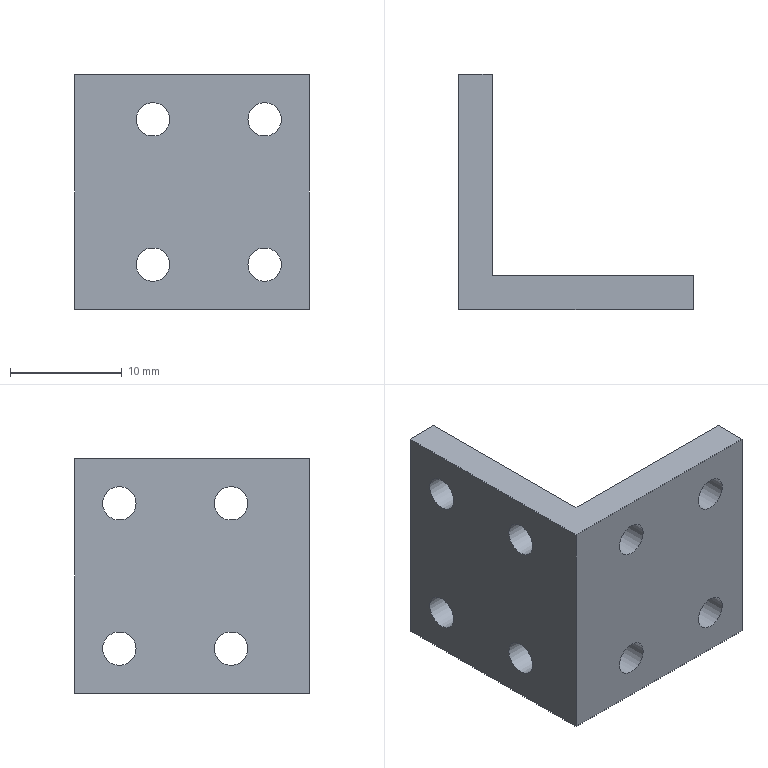Part | STEP file | 1-01.5 | 1 solid | 16 faces | box 21 x 21 x 21 mm | volume 2287 mm3 | plane 8 | cylinder 8 | commonest cylinder face diameters 3 x8
STEP:
#1=CARTESIAN_POINT('',(0.,0.,0.));
#2=DIRECTION('',(0.,0.,1.));
#3=DIRECTION('',(1.,0.,0.));
#4=AXIS2_PLACEMENT_3D('',#1,#2,#3);
#5=CARTESIAN_POINT('',(-3.,-10.5,-10.5));
#6=VERTEX_POINT('',#5);
#7=CARTESIAN_POINT('',(-3.,10.5,-10.5));
#8=VERTEX_POINT('',#7);
#9=CARTESIAN_POINT('',(-3.,-10.5,-10.5));
#10=DIRECTION('',(0.,1.,0.));
#11=VECTOR('',#10,1.);
#12=LINE('',#9,#11);
#13=CARTESIAN_POINT('',(-3.,0.,0.));
#14=DIRECTION('',(1.,0.,0.));
#15=DIRECTION('',(0.,1.,0.));
#16=AXIS2_PLACEMENT_3D('',#13,#14,#15);
#17=PLANE('',#16);
#18=CARTESIAN_POINT('',(-10.5,-10.5));
#19=DIRECTION('',(1.,0.));
#20=VECTOR('',#19,1.);
#21=LINE('',#18,#20);
#22=(GEOMETRIC_REPRESENTATION_CONTEXT(2)PARAMETRIC_REPRESENTATION_CONTEXT()REPRESENTATION_CONTEXT('',''));
#23=DEFINITIONAL_REPRESENTATION('',(#21),#22);
#24=PCURVE('',#17,#23);
#25=CARTESIAN_POINT('',(7.5,0.,-10.5));
#26=DIRECTION('',(0.,0.,1.));
#27=DIRECTION('',(0.,1.,0.));
#28=AXIS2_PLACEMENT_3D('',#25,#26,#27);
#29=PLANE('',#28);
#30=CARTESIAN_POINT('',(-10.5,10.5));
#31=DIRECTION('',(1.,0.));
#32=VECTOR('',#31,1.);
#33=LINE('',#30,#32);
#34=(GEOMETRIC_REPRESENTATION_CONTEXT(2)PARAMETRIC_REPRESENTATION_CONTEXT()REPRESENTATION_CONTEXT('',''));
#35=DEFINITIONAL_REPRESENTATION('',(#33),#34);
#36=PCURVE('',#29,#35);
#37=SURFACE_CURVE('',#12,(#24,#36),.PCURVE_S1.);
#38=EDGE_CURVE('',#6,#8,#37,.T.);
#39=ORIENTED_EDGE('',*,*,#38,.T.);
#40=CARTESIAN_POINT('',(-3.,10.5,10.5));
#41=VERTEX_POINT('',#40);
#42=CARTESIAN_POINT('',(-3.,10.5,-10.5));
#43=DIRECTION('',(0.,0.,1.));
#44=VECTOR('',#43,1.);
#45=LINE('',#42,#44);
#46=CARTESIAN_POINT('',(10.5,-10.5));
#47=DIRECTION('',(0.,1.));
#48=VECTOR('',#47,1.);
#49=LINE('',#46,#48);
#50=(GEOMETRIC_REPRESENTATION_CONTEXT(2)PARAMETRIC_REPRESENTATION_CONTEXT()REPRESENTATION_CONTEXT('',''));
#51=DEFINITIONAL_REPRESENTATION('',(#49),#50);
#52=PCURVE('',#17,#51);
#53=CARTESIAN_POINT('',(-1.5,10.5,0.));
#54=DIRECTION('',(0.,-1.,0.));
#55=DIRECTION('',(0.,0.,1.));
#56=AXIS2_PLACEMENT_3D('',#53,#54,#55);
#57=PLANE('',#56);
#58=CARTESIAN_POINT('',(-10.5,1.5));
#59=DIRECTION('',(1.,0.));
#60=VECTOR('',#59,1.);
#61=LINE('',#58,#60);
#62=(GEOMETRIC_REPRESENTATION_CONTEXT(2)PARAMETRIC_REPRESENTATION_CONTEXT()REPRESENTATION_CONTEXT('',''));
#63=DEFINITIONAL_REPRESENTATION('',(#61),#62);
#64=PCURVE('',#57,#63);
#65=SURFACE_CURVE('',#45,(#52,#64),.PCURVE_S1.);
#66=EDGE_CURVE('',#8,#41,#65,.T.);
#67=ORIENTED_EDGE('',*,*,#66,.T.);
#68=CARTESIAN_POINT('',(-3.,-10.5,10.5));
#69=VERTEX_POINT('',#68);
#70=CARTESIAN_POINT('',(-3.,10.5,10.5));
#71=DIRECTION('',(0.,-1.,0.));
#72=VECTOR('',#71,1.);
#73=LINE('',#70,#72);
#74=CARTESIAN_POINT('',(10.5,10.5));
#75=DIRECTION('',(-1.,0.));
#76=VECTOR('',#75,1.);
#77=LINE('',#74,#76);
#78=(GEOMETRIC_REPRESENTATION_CONTEXT(2)PARAMETRIC_REPRESENTATION_CONTEXT()REPRESENTATION_CONTEXT('',''));
#79=DEFINITIONAL_REPRESENTATION('',(#77),#78);
#80=PCURVE('',#17,#79);
#81=CARTESIAN_POINT('',(7.5,0.,10.5));
#82=DIRECTION('',(0.,0.,-1.));
#83=DIRECTION('',(0.,-1.,0.));
#84=AXIS2_PLACEMENT_3D('',#81,#82,#83);
#85=PLANE('',#84);
#86=CARTESIAN_POINT('',(-10.5,10.5));
#87=DIRECTION('',(1.,0.));
#88=VECTOR('',#87,1.);
#89=LINE('',#86,#88);
#90=(GEOMETRIC_REPRESENTATION_CONTEXT(2)PARAMETRIC_REPRESENTATION_CONTEXT()REPRESENTATION_CONTEXT('',''));
#91=DEFINITIONAL_REPRESENTATION('',(#89),#90);
#92=PCURVE('',#85,#91);
#93=SURFACE_CURVE('',#73,(#80,#92),.PCURVE_S1.);
#94=EDGE_CURVE('',#41,#69,#93,.T.);
#95=ORIENTED_EDGE('',*,*,#94,.T.);
#96=CARTESIAN_POINT('',(-3.,-10.5,10.5));
#97=DIRECTION('',(0.,0.,-1.));
#98=VECTOR('',#97,1.);
#99=LINE('',#96,#98);
#100=CARTESIAN_POINT('',(-10.5,10.5));
#101=DIRECTION('',(0.,-1.));
#102=VECTOR('',#101,1.);
#103=LINE('',#100,#102);
#104=(GEOMETRIC_REPRESENTATION_CONTEXT(2)PARAMETRIC_REPRESENTATION_CONTEXT()REPRESENTATION_CONTEXT('',''));
#105=DEFINITIONAL_REPRESENTATION('',(#103),#104);
#106=PCURVE('',#17,#105);
#107=CARTESIAN_POINT('',(9.525,-10.5,0.));
#108=DIRECTION('',(0.,1.,0.));
#109=DIRECTION('',(0.,0.,-1.));
#110=AXIS2_PLACEMENT_3D('',#107,#108,#109);
#111=PLANE('',#110);
#112=CARTESIAN_POINT('',(-10.5,12.525));
#113=DIRECTION('',(1.,0.));
#114=VECTOR('',#113,1.);
#115=LINE('',#112,#114);
#116=(GEOMETRIC_REPRESENTATION_CONTEXT(2)PARAMETRIC_REPRESENTATION_CONTEXT()REPRESENTATION_CONTEXT('',''));
#117=DEFINITIONAL_REPRESENTATION('',(#115),#116);
#118=PCURVE('',#111,#117);
#119=SURFACE_CURVE('',#99,(#106,#118),.PCURVE_S1.);
#120=EDGE_CURVE('',#69,#6,#119,.T.);
#121=ORIENTED_EDGE('',*,*,#120,.T.);
#122=EDGE_LOOP('',(#39,#67,#95,#121));
#123=FACE_BOUND('',#122,.F.);
#124=CARTESIAN_POINT('',(-3.,8.,6.5));
#125=VERTEX_POINT('',#124);
#126=CARTESIAN_POINT('',(-3.,6.5,6.5));
#127=DIRECTION('',(-1.,0.,0.));
#128=DIRECTION('',(0.,1.,0.));
#129=AXIS2_PLACEMENT_3D('',#126,#127,#128);
#130=CIRCLE('',#129,1.5);
#131=CARTESIAN_POINT('',(8.,6.5));
#132=CARTESIAN_POINT('',(8.,3.902));
#133=CARTESIAN_POINT('',(5.75,5.201));
#134=CARTESIAN_POINT('',(3.5,6.5));
#135=CARTESIAN_POINT('',(5.75,7.799));
#136=CARTESIAN_POINT('',(8.,9.098));
#137=CARTESIAN_POINT('',(8.,6.5));
#138=(BOUNDED_CURVE()B_SPLINE_CURVE(2,(#131,#132,#133,#134,#135,#136,#137),.UNSPECIFIED.,.T.,.F.)B_SPLINE_CURVE_WITH_KNOTS((1,2,2,2,2,1),(-2.094,0.,2.094,4.189,6.283,8.378),.UNSPECIFIED.)CURVE()GEOMETRIC_REPRESENTATION_ITEM()RATIONAL_B_SPLINE_CURVE((1.,0.5,1.,0.5,1.,0.5,1.))REPRESENTATION_ITEM(''));
#139=(GEOMETRIC_REPRESENTATION_CONTEXT(2)PARAMETRIC_REPRESENTATION_CONTEXT()REPRESENTATION_CONTEXT('',''));
#140=DEFINITIONAL_REPRESENTATION('',(#138),#139);
#141=PCURVE('',#17,#140);
#142=CARTESIAN_POINT('',(0.,6.5,6.5));
#143=DIRECTION('',(-1.,0.,0.));
#144=DIRECTION('',(0.,1.,0.));
#145=AXIS2_PLACEMENT_3D('',#142,#143,#144);
#146=CYLINDRICAL_SURFACE('',#145,1.5);
#147=CARTESIAN_POINT('',(0.,3.));
#148=DIRECTION('',(1.,0.));
#149=VECTOR('',#148,1.);
#150=LINE('',#147,#149);
#151=(GEOMETRIC_REPRESENTATION_CONTEXT(2)PARAMETRIC_REPRESENTATION_CONTEXT()REPRESENTATION_CONTEXT('',''));
#152=DEFINITIONAL_REPRESENTATION('',(#150),#151);
#153=PCURVE('',#146,#152);
#154=SURFACE_CURVE('',#130,(#141,#153),.PCURVE_S1.);
#155=EDGE_CURVE('',#125,#125,#154,.T.);
#156=ORIENTED_EDGE('',*,*,#155,.T.);
#157=EDGE_LOOP('',(#156));
#158=FACE_BOUND('',#157,.F.);
#159=CARTESIAN_POINT('',(-3.,8.,-6.5));
#160=VERTEX_POINT('',#159);
#161=CARTESIAN_POINT('',(-3.,6.5,-6.5));
#162=DIRECTION('',(-1.,0.,0.));
#163=DIRECTION('',(0.,1.,0.));
#164=AXIS2_PLACEMENT_3D('',#161,#162,#163);
#165=CIRCLE('',#164,1.5);
#166=CARTESIAN_POINT('',(8.,-6.5));
#167=CARTESIAN_POINT('',(8.,-9.098));
#168=CARTESIAN_POINT('',(5.75,-7.799));
#169=CARTESIAN_POINT('',(3.5,-6.5));
#170=CARTESIAN_POINT('',(5.75,-5.201));
#171=CARTESIAN_POINT('',(8.,-3.902));
#172=CARTESIAN_POINT('',(8.,-6.5));
#173=(BOUNDED_CURVE()B_SPLINE_CURVE(2,(#166,#167,#168,#169,#170,#171,#172),.UNSPECIFIED.,.T.,.F.)B_SPLINE_CURVE_WITH_KNOTS((1,2,2,2,2,1),(-2.094,0.,2.094,4.189,6.283,8.378),.UNSPECIFIED.)CURVE()GEOMETRIC_REPRESENTATION_ITEM()RATIONAL_B_SPLINE_CURVE((1.,0.5,1.,0.5,1.,0.5,1.))REPRESENTATION_ITEM(''));
#174=(GEOMETRIC_REPRESENTATION_CONTEXT(2)PARAMETRIC_REPRESENTATION_CONTEXT()REPRESENTATION_CONTEXT('',''));
#175=DEFINITIONAL_REPRESENTATION('',(#173),#174);
#176=PCURVE('',#17,#175);
#177=CARTESIAN_POINT('',(0.,6.5,-6.5));
#178=DIRECTION('',(-1.,0.,0.));
#179=DIRECTION('',(0.,1.,0.));
#180=AXIS2_PLACEMENT_3D('',#177,#178,#179);
#181=CYLINDRICAL_SURFACE('',#180,1.5);
#182=CARTESIAN_POINT('',(0.,3.));
#183=DIRECTION('',(1.,0.));
#184=VECTOR('',#183,1.);
#185=LINE('',#182,#184);
#186=(GEOMETRIC_REPRESENTATION_CONTEXT(2)PARAMETRIC_REPRESENTATION_CONTEXT()REPRESENTATION_CONTEXT('',''));
#187=DEFINITIONAL_REPRESENTATION('',(#185),#186);
#188=PCURVE('',#181,#187);
#189=SURFACE_CURVE('',#165,(#176,#188),.PCURVE_S1.);
#190=EDGE_CURVE('',#160,#160,#189,.T.);
#191=ORIENTED_EDGE('',*,*,#190,.T.);
#192=EDGE_LOOP('',(#191));
#193=FACE_BOUND('',#192,.F.);
#194=CARTESIAN_POINT('',(-3.,-2.,-6.5));
#195=VERTEX_POINT('',#194);
#196=CARTESIAN_POINT('',(-3.,-3.5,-6.5));
#197=DIRECTION('',(-1.,0.,0.));
#198=DIRECTION('',(0.,1.,0.));
#199=AXIS2_PLACEMENT_3D('',#196,#197,#198);
#200=CIRCLE('',#199,1.5);
#201=CARTESIAN_POINT('',(-2.,-6.5));
#202=CARTESIAN_POINT('',(-2.,-9.098));
#203=CARTESIAN_POINT('',(-4.25,-7.799));
#204=CARTESIAN_POINT('',(-6.5,-6.5));
#205=CARTESIAN_POINT('',(-4.25,-5.201));
#206=CARTESIAN_POINT('',(-2.,-3.902));
#207=CARTESIAN_POINT('',(-2.,-6.5));
#208=(BOUNDED_CURVE()B_SPLINE_CURVE(2,(#201,#202,#203,#204,#205,#206,#207),.UNSPECIFIED.,.T.,.F.)B_SPLINE_CURVE_WITH_KNOTS((1,2,2,2,2,1),(-2.094,0.,2.094,4.189,6.283,8.378),.UNSPECIFIED.)CURVE()GEOMETRIC_REPRESENTATION_ITEM()RATIONAL_B_SPLINE_CURVE((1.,0.5,1.,0.5,1.,0.5,1.))REPRESENTATION_ITEM(''));
#209=(GEOMETRIC_REPRESENTATION_CONTEXT(2)PARAMETRIC_REPRESENTATION_CONTEXT()REPRESENTATION_CONTEXT('',''));
#210=DEFINITIONAL_REPRESENTATION('',(#208),#209);
#211=PCURVE('',#17,#210);
#212=CARTESIAN_POINT('',(0.,-3.5,-6.5));
#213=DIRECTION('',(-1.,0.,0.));
#214=DIRECTION('',(0.,1.,0.));
#215=AXIS2_PLACEMENT_3D('',#212,#213,#214);
#216=CYLINDRICAL_SURFACE('',#215,1.5);
#217=CARTESIAN_POINT('',(0.,3.));
#218=DIRECTION('',(1.,0.));
#219=VECTOR('',#218,1.);
#220=LINE('',#217,#219);
#221=(GEOMETRIC_REPRESENTATION_CONTEXT(2)PARAMETRIC_REPRESENTATION_CONTEXT()REPRESENTATION_CONTEXT('',''));
#222=DEFINITIONAL_REPRESENTATION('',(#220),#221);
#223=PCURVE('',#216,#222);
#224=SURFACE_CURVE('',#200,(#211,#223),.PCURVE_S1.);
#225=EDGE_CURVE('',#195,#195,#224,.T.);
#226=ORIENTED_EDGE('',*,*,#225,.T.);
#227=EDGE_LOOP('',(#226));
#228=FACE_BOUND('',#227,.F.);
#229=CARTESIAN_POINT('',(-3.,-2.,6.5));
#230=VERTEX_POINT('',#229);
#231=CARTESIAN_POINT('',(-3.,-3.5,6.5));
#232=DIRECTION('',(-1.,0.,0.));
#233=DIRECTION('',(0.,1.,0.));
#234=AXIS2_PLACEMENT_3D('',#231,#232,#233);
#235=CIRCLE('',#234,1.5);
#236=CARTESIAN_POINT('',(-2.,6.5));
#237=CARTESIAN_POINT('',(-2.,3.902));
#238=CARTESIAN_POINT('',(-4.25,5.201));
#239=CARTESIAN_POINT('',(-6.5,6.5));
#240=CARTESIAN_POINT('',(-4.25,7.799));
#241=CARTESIAN_POINT('',(-2.,9.098));
#242=CARTESIAN_POINT('',(-2.,6.5));
#243=(BOUNDED_CURVE()B_SPLINE_CURVE(2,(#236,#237,#238,#239,#240,#241,#242),.UNSPECIFIED.,.T.,.F.)B_SPLINE_CURVE_WITH_KNOTS((1,2,2,2,2,1),(-2.094,0.,2.094,4.189,6.283,8.378),.UNSPECIFIED.)CURVE()GEOMETRIC_REPRESENTATION_ITEM()RATIONAL_B_SPLINE_CURVE((1.,0.5,1.,0.5,1.,0.5,1.))REPRESENTATION_ITEM(''));
#244=(GEOMETRIC_REPRESENTATION_CONTEXT(2)PARAMETRIC_REPRESENTATION_CONTEXT()REPRESENTATION_CONTEXT('',''));
#245=DEFINITIONAL_REPRESENTATION('',(#243),#244);
#246=PCURVE('',#17,#245);
#247=CARTESIAN_POINT('',(0.,-3.5,6.5));
#248=DIRECTION('',(-1.,0.,0.));
#249=DIRECTION('',(0.,1.,0.));
#250=AXIS2_PLACEMENT_3D('',#247,#248,#249);
#251=CYLINDRICAL_SURFACE('',#250,1.5);
#252=CARTESIAN_POINT('',(0.,3.));
#253=DIRECTION('',(1.,0.));
#254=VECTOR('',#253,1.);
#255=LINE('',#252,#254);
#256=(GEOMETRIC_REPRESENTATION_CONTEXT(2)PARAMETRIC_REPRESENTATION_CONTEXT()REPRESENTATION_CONTEXT('',''));
#257=DEFINITIONAL_REPRESENTATION('',(#255),#256);
#258=PCURVE('',#251,#257);
#259=SURFACE_CURVE('',#235,(#246,#258),.PCURVE_S1.);
#260=EDGE_CURVE('',#230,#230,#259,.T.);
#261=ORIENTED_EDGE('',*,*,#260,.T.);
#262=EDGE_LOOP('',(#261));
#263=FACE_BOUND('',#262,.F.);
#264=ADVANCED_FACE('',(#123,#158,#193,#228,#263),#17,.F.);
#265=CARTESIAN_POINT('',(0.,-7.5,-10.5));
#266=VERTEX_POINT('',#265);
#267=CARTESIAN_POINT('',(0.,10.5,-10.5));
#268=VERTEX_POINT('',#267);
#269=CARTESIAN_POINT('',(0.,-7.5,-10.5));
#270=DIRECTION('',(0.,1.,0.));
#271=VECTOR('',#270,1.);
#272=LINE('',#269,#271);
#273=CARTESIAN_POINT('',(-7.5,7.5));
#274=DIRECTION('',(1.,0.));
#275=VECTOR('',#274,1.);
#276=LINE('',#273,#275);
#277=(GEOMETRIC_REPRESENTATION_CONTEXT(2)PARAMETRIC_REPRESENTATION_CONTEXT()REPRESENTATION_CONTEXT('',''));
#278=DEFINITIONAL_REPRESENTATION('',(#276),#277);
#279=PCURVE('',#29,#278);
#280=CARTESIAN_POINT('',(0.,0.,0.));
#281=DIRECTION('',(1.,0.,0.));
#282=DIRECTION('',(0.,1.,0.));
#283=AXIS2_PLACEMENT_3D('',#280,#281,#282);
#284=PLANE('',#283);
#285=CARTESIAN_POINT('',(-7.5,-10.5));
#286=DIRECTION('',(1.,0.));
#287=VECTOR('',#286,1.);
#288=LINE('',#285,#287);
#289=(GEOMETRIC_REPRESENTATION_CONTEXT(2)PARAMETRIC_REPRESENTATION_CONTEXT()REPRESENTATION_CONTEXT('',''));
#290=DEFINITIONAL_REPRESENTATION('',(#288),#289);
#291=PCURVE('',#284,#290);
#292=SURFACE_CURVE('',#272,(#279,#291),.PCURVE_S1.);
#293=EDGE_CURVE('',#266,#268,#292,.T.);
#294=ORIENTED_EDGE('',*,*,#293,.T.);
#295=CARTESIAN_POINT('',(0.,10.5,-10.5));
#296=DIRECTION('',(-1.,0.,0.));
#297=VECTOR('',#296,1.);
#298=LINE('',#295,#297);
#299=CARTESIAN_POINT('',(10.5,7.5));
#300=DIRECTION('',(0.,1.));
#301=VECTOR('',#300,1.);
#302=LINE('',#299,#301);
#303=(GEOMETRIC_REPRESENTATION_CONTEXT(2)PARAMETRIC_REPRESENTATION_CONTEXT()REPRESENTATION_CONTEXT('',''));
#304=DEFINITIONAL_REPRESENTATION('',(#302),#303);
#305=PCURVE('',#29,#304);
#306=CARTESIAN_POINT('',(-10.5,-1.5));
#307=DIRECTION('',(0.,1.));
#308=VECTOR('',#307,1.);
#309=LINE('',#306,#308);
#310=(GEOMETRIC_REPRESENTATION_CONTEXT(2)PARAMETRIC_REPRESENTATION_CONTEXT()REPRESENTATION_CONTEXT('',''));
#311=DEFINITIONAL_REPRESENTATION('',(#309),#310);
#312=PCURVE('',#57,#311);
#313=SURFACE_CURVE('',#298,(#305,#312),.PCURVE_S1.);
#314=EDGE_CURVE('',#268,#8,#313,.T.);
#315=ORIENTED_EDGE('',*,*,#314,.T.);
#316=ORIENTED_EDGE('',*,*,#38,.F.);
#317=CARTESIAN_POINT('',(18.,-10.5,-10.5));
#318=VERTEX_POINT('',#317);
#319=CARTESIAN_POINT('',(18.,-10.5,-10.5));
#320=DIRECTION('',(-1.,0.,0.));
#321=VECTOR('',#320,1.);
#322=LINE('',#319,#321);
#323=CARTESIAN_POINT('',(-10.5,-10.5));
#324=DIRECTION('',(0.,1.));
#325=VECTOR('',#324,1.);
#326=LINE('',#323,#325);
#327=(GEOMETRIC_REPRESENTATION_CONTEXT(2)PARAMETRIC_REPRESENTATION_CONTEXT()REPRESENTATION_CONTEXT('',''));
#328=DEFINITIONAL_REPRESENTATION('',(#326),#327);
#329=PCURVE('',#29,#328);
#330=CARTESIAN_POINT('',(10.5,-8.475));
#331=DIRECTION('',(0.,1.));
#332=VECTOR('',#331,1.);
#333=LINE('',#330,#332);
#334=(GEOMETRIC_REPRESENTATION_CONTEXT(2)PARAMETRIC_REPRESENTATION_CONTEXT()REPRESENTATION_CONTEXT('',''));
#335=DEFINITIONAL_REPRESENTATION('',(#333),#334);
#336=PCURVE('',#111,#335);
#337=SURFACE_CURVE('',#322,(#329,#336),.PCURVE_S1.);
#338=EDGE_CURVE('',#318,#6,#337,.T.);
#339=ORIENTED_EDGE('',*,*,#338,.F.);
#340=CARTESIAN_POINT('',(18.,-7.5,-10.5));
#341=VERTEX_POINT('',#340);
#342=CARTESIAN_POINT('',(18.,-10.5,-10.5));
#343=DIRECTION('',(0.,1.,0.));
#344=VECTOR('',#343,1.);
#345=LINE('',#342,#344);
#346=CARTESIAN_POINT('',(-10.5,-10.5));
#347=DIRECTION('',(1.,0.));
#348=VECTOR('',#347,1.);
#349=LINE('',#346,#348);
#350=(GEOMETRIC_REPRESENTATION_CONTEXT(2)PARAMETRIC_REPRESENTATION_CONTEXT()REPRESENTATION_CONTEXT('',''));
#351=DEFINITIONAL_REPRESENTATION('',(#349),#350);
#352=PCURVE('',#29,#351);
#353=CARTESIAN_POINT('',(18.,-9.,0.));
#354=DIRECTION('',(-1.,0.,0.));
#355=DIRECTION('',(0.,0.,1.));
#356=AXIS2_PLACEMENT_3D('',#353,#354,#355);
#357=PLANE('',#356);
#358=CARTESIAN_POINT('',(-10.5,-1.5));
#359=DIRECTION('',(0.,1.));
#360=VECTOR('',#359,1.);
#361=LINE('',#358,#360);
#362=(GEOMETRIC_REPRESENTATION_CONTEXT(2)PARAMETRIC_REPRESENTATION_CONTEXT()REPRESENTATION_CONTEXT('',''));
#363=DEFINITIONAL_REPRESENTATION('',(#361),#362);
#364=PCURVE('',#357,#363);
#365=SURFACE_CURVE('',#345,(#352,#364),.PCURVE_S1.);
#366=EDGE_CURVE('',#318,#341,#365,.T.);
#367=ORIENTED_EDGE('',*,*,#366,.T.);
#368=CARTESIAN_POINT('',(0.,-7.5,-10.5));
#369=DIRECTION('',(1.,0.,0.));
#370=VECTOR('',#369,1.);
#371=LINE('',#368,#370);
#372=CARTESIAN_POINT('',(-7.5,7.5));
#373=DIRECTION('',(0.,-1.));
#374=VECTOR('',#373,1.);
#375=LINE('',#372,#374);
#376=(GEOMETRIC_REPRESENTATION_CONTEXT(2)PARAMETRIC_REPRESENTATION_CONTEXT()REPRESENTATION_CONTEXT('',''));
#377=DEFINITIONAL_REPRESENTATION('',(#375),#376);
#378=PCURVE('',#29,#377);
#379=CARTESIAN_POINT('',(10.5,-7.5,0.));
#380=DIRECTION('',(0.,-1.,0.));
#381=DIRECTION('',(1.,0.,0.));
#382=AXIS2_PLACEMENT_3D('',#379,#380,#381);
#383=PLANE('',#382);
#384=CARTESIAN_POINT('',(-10.5,-10.5));
#385=DIRECTION('',(1.,0.));
#386=VECTOR('',#385,1.);
#387=LINE('',#384,#386);
#388=(GEOMETRIC_REPRESENTATION_CONTEXT(2)PARAMETRIC_REPRESENTATION_CONTEXT()REPRESENTATION_CONTEXT('',''));
#389=DEFINITIONAL_REPRESENTATION('',(#387),#388);
#390=PCURVE('',#383,#389);
#391=SURFACE_CURVE('',#371,(#378,#390),.PCURVE_S1.);
#392=EDGE_CURVE('',#266,#341,#391,.T.);
#393=ORIENTED_EDGE('',*,*,#392,.F.);
#394=EDGE_LOOP('',(#294,#315,#316,#339,#367,#393));
#395=FACE_BOUND('',#394,.F.);
#396=ADVANCED_FACE('',(#395),#29,.F.);
#397=CARTESIAN_POINT('',(0.,10.5,10.5));
#398=VERTEX_POINT('',#397);
#399=CARTESIAN_POINT('',(0.,10.5,-10.5));
#400=DIRECTION('',(0.,0.,1.));
#401=VECTOR('',#400,1.);
#402=LINE('',#399,#401);
#403=CARTESIAN_POINT('',(-10.5,-1.5));
#404=DIRECTION('',(1.,0.));
#405=VECTOR('',#404,1.);
#406=LINE('',#403,#405);
#407=(GEOMETRIC_REPRESENTATION_CONTEXT(2)PARAMETRIC_REPRESENTATION_CONTEXT()REPRESENTATION_CONTEXT('',''));
#408=DEFINITIONAL_REPRESENTATION('',(#406),#407);
#409=PCURVE('',#57,#408);
#410=CARTESIAN_POINT('',(10.5,-10.5));
#411=DIRECTION('',(0.,1.));
#412=VECTOR('',#411,1.);
#413=LINE('',#410,#412);
#414=(GEOMETRIC_REPRESENTATION_CONTEXT(2)PARAMETRIC_REPRESENTATION_CONTEXT()REPRESENTATION_CONTEXT('',''));
#415=DEFINITIONAL_REPRESENTATION('',(#413),#414);
#416=PCURVE('',#284,#415);
#417=SURFACE_CURVE('',#402,(#409,#416),.PCURVE_S1.);
#418=EDGE_CURVE('',#268,#398,#417,.T.);
#419=ORIENTED_EDGE('',*,*,#418,.T.);
#420=CARTESIAN_POINT('',(0.,10.5,10.5));
#421=DIRECTION('',(-1.,0.,0.));
#422=VECTOR('',#421,1.);
#423=LINE('',#420,#422);
#424=CARTESIAN_POINT('',(10.5,-1.5));
#425=DIRECTION('',(0.,1.));
#426=VECTOR('',#425,1.);
#427=LINE('',#424,#426);
#428=(GEOMETRIC_REPRESENTATION_CONTEXT(2)PARAMETRIC_REPRESENTATION_CONTEXT()REPRESENTATION_CONTEXT('',''));
#429=DEFINITIONAL_REPRESENTATION('',(#427),#428);
#430=PCURVE('',#57,#429);
#431=CARTESIAN_POINT('',(-10.5,7.5));
#432=DIRECTION('',(0.,1.));
#433=VECTOR('',#432,1.);
#434=LINE('',#431,#433);
#435=(GEOMETRIC_REPRESENTATION_CONTEXT(2)PARAMETRIC_REPRESENTATION_CONTEXT()REPRESENTATION_CONTEXT('',''));
#436=DEFINITIONAL_REPRESENTATION('',(#434),#435);
#437=PCURVE('',#85,#436);
#438=SURFACE_CURVE('',#423,(#430,#437),.PCURVE_S1.);
#439=EDGE_CURVE('',#398,#41,#438,.T.);
#440=ORIENTED_EDGE('',*,*,#439,.T.);
#441=ORIENTED_EDGE('',*,*,#66,.F.);
#442=ORIENTED_EDGE('',*,*,#314,.F.);
#443=EDGE_LOOP('',(#419,#440,#441,#442));
#444=FACE_BOUND('',#443,.F.);
#445=ADVANCED_FACE('',(#444),#57,.F.);
#446=ORIENTED_EDGE('',*,*,#94,.F.);
#447=ORIENTED_EDGE('',*,*,#439,.F.);
#448=CARTESIAN_POINT('',(0.,-7.5,10.5));
#449=VERTEX_POINT('',#448);
#450=CARTESIAN_POINT('',(0.,10.5,10.5));
#451=DIRECTION('',(0.,-1.,0.));
#452=VECTOR('',#451,1.);
#453=LINE('',#450,#452);
#454=CARTESIAN_POINT('',(-10.5,7.5));
#455=DIRECTION('',(1.,0.));
#456=VECTOR('',#455,1.);
#457=LINE('',#454,#456);
#458=(GEOMETRIC_REPRESENTATION_CONTEXT(2)PARAMETRIC_REPRESENTATION_CONTEXT()REPRESENTATION_CONTEXT('',''));
#459=DEFINITIONAL_REPRESENTATION('',(#457),#458);
#460=PCURVE('',#85,#459);
#461=CARTESIAN_POINT('',(10.5,10.5));
#462=DIRECTION('',(-1.,0.));
#463=VECTOR('',#462,1.);
#464=LINE('',#461,#463);
#465=(GEOMETRIC_REPRESENTATION_CONTEXT(2)PARAMETRIC_REPRESENTATION_CONTEXT()REPRESENTATION_CONTEXT('',''));
#466=DEFINITIONAL_REPRESENTATION('',(#464),#465);
#467=PCURVE('',#284,#466);
#468=SURFACE_CURVE('',#453,(#460,#467),.PCURVE_S1.);
#469=EDGE_CURVE('',#398,#449,#468,.T.);
#470=ORIENTED_EDGE('',*,*,#469,.T.);
#471=CARTESIAN_POINT('',(18.,-7.5,10.5));
#472=VERTEX_POINT('',#471);
#473=CARTESIAN_POINT('',(18.,-7.5,10.5));
#474=DIRECTION('',(-1.,0.,0.));
#475=VECTOR('',#474,1.);
#476=LINE('',#473,#475);
#477=CARTESIAN_POINT('',(7.5,-10.5));
#478=DIRECTION('',(0.,1.));
#479=VECTOR('',#478,1.);
#480=LINE('',#477,#479);
#481=(GEOMETRIC_REPRESENTATION_CONTEXT(2)PARAMETRIC_REPRESENTATION_CONTEXT()REPRESENTATION_CONTEXT('',''));
#482=DEFINITIONAL_REPRESENTATION('',(#480),#481);
#483=PCURVE('',#85,#482);
#484=CARTESIAN_POINT('',(7.5,10.5));
#485=DIRECTION('',(-1.,0.));
#486=VECTOR('',#485,1.);
#487=LINE('',#484,#486);
#488=(GEOMETRIC_REPRESENTATION_CONTEXT(2)PARAMETRIC_REPRESENTATION_CONTEXT()REPRESENTATION_CONTEXT('',''));
#489=DEFINITIONAL_REPRESENTATION('',(#487),#488);
#490=PCURVE('',#383,#489);
#491=SURFACE_CURVE('',#476,(#483,#490),.PCURVE_S1.);
#492=EDGE_CURVE('',#472,#449,#491,.T.);
#493=ORIENTED_EDGE('',*,*,#492,.F.);
#494=CARTESIAN_POINT('',(18.,-10.5,10.5));
#495=VERTEX_POINT('',#494);
#496=CARTESIAN_POINT('',(18.,-10.5,10.5));
#497=DIRECTION('',(0.,1.,0.));
#498=VECTOR('',#497,1.);
#499=LINE('',#496,#498);
#500=CARTESIAN_POINT('',(10.5,-10.5));
#501=DIRECTION('',(-1.,0.));
#502=VECTOR('',#501,1.);
#503=LINE('',#500,#502);
#504=(GEOMETRIC_REPRESENTATION_CONTEXT(2)PARAMETRIC_REPRESENTATION_CONTEXT()REPRESENTATION_CONTEXT('',''));
#505=DEFINITIONAL_REPRESENTATION('',(#503),#504);
#506=PCURVE('',#85,#505);
#507=CARTESIAN_POINT('',(10.5,-1.5));
#508=DIRECTION('',(0.,1.));
#509=VECTOR('',#508,1.);
#510=LINE('',#507,#509);
#511=(GEOMETRIC_REPRESENTATION_CONTEXT(2)PARAMETRIC_REPRESENTATION_CONTEXT()REPRESENTATION_CONTEXT('',''));
#512=DEFINITIONAL_REPRESENTATION('',(#510),#511);
#513=PCURVE('',#357,#512);
#514=SURFACE_CURVE('',#499,(#506,#513),.PCURVE_S1.);
#515=EDGE_CURVE('',#495,#472,#514,.T.);
#516=ORIENTED_EDGE('',*,*,#515,.F.);
#517=CARTESIAN_POINT('',(-3.,-10.5,10.5));
#518=DIRECTION('',(1.,0.,0.));
#519=VECTOR('',#518,1.);
#520=LINE('',#517,#519);
#521=CARTESIAN_POINT('',(10.5,10.5));
#522=DIRECTION('',(0.,-1.));
#523=VECTOR('',#522,1.);
#524=LINE('',#521,#523);
#525=(GEOMETRIC_REPRESENTATION_CONTEXT(2)PARAMETRIC_REPRESENTATION_CONTEXT()REPRESENTATION_CONTEXT('',''));
#526=DEFINITIONAL_REPRESENTATION('',(#524),#525);
#527=PCURVE('',#85,#526);
#528=CARTESIAN_POINT('',(-10.5,12.525));
#529=DIRECTION('',(0.,-1.));
#530=VECTOR('',#529,1.);
#531=LINE('',#528,#530);
#532=(GEOMETRIC_REPRESENTATION_CONTEXT(2)PARAMETRIC_REPRESENTATION_CONTEXT()REPRESENTATION_CONTEXT('',''));
#533=DEFINITIONAL_REPRESENTATION('',(#531),#532);
#534=PCURVE('',#111,#533);
#535=SURFACE_CURVE('',#520,(#527,#534),.PCURVE_S1.);
#536=EDGE_CURVE('',#69,#495,#535,.T.);
#537=ORIENTED_EDGE('',*,*,#536,.F.);
#538=EDGE_LOOP('',(#446,#447,#470,#493,#516,#537));
#539=FACE_BOUND('',#538,.F.);
#540=ADVANCED_FACE('',(#539),#85,.F.);
#541=ORIENTED_EDGE('',*,*,#120,.F.);
#542=ORIENTED_EDGE('',*,*,#536,.T.);
#543=CARTESIAN_POINT('',(18.,-10.5,-10.5));
#544=DIRECTION('',(0.,0.,1.));
#545=VECTOR('',#544,1.);
#546=LINE('',#543,#545);
#547=CARTESIAN_POINT('',(10.5,-8.475));
#548=DIRECTION('',(-1.,0.));
#549=VECTOR('',#548,1.);
#550=LINE('',#547,#549);
#551=(GEOMETRIC_REPRESENTATION_CONTEXT(2)PARAMETRIC_REPRESENTATION_CONTEXT()REPRESENTATION_CONTEXT('',''));
#552=DEFINITIONAL_REPRESENTATION('',(#550),#551);
#553=PCURVE('',#111,#552);
#554=CARTESIAN_POINT('',(-10.5,-1.5));
#555=DIRECTION('',(1.,0.));
#556=VECTOR('',#555,1.);
#557=LINE('',#554,#556);
#558=(GEOMETRIC_REPRESENTATION_CONTEXT(2)PARAMETRIC_REPRESENTATION_CONTEXT()REPRESENTATION_CONTEXT('',''));
#559=DEFINITIONAL_REPRESENTATION('',(#557),#558);
#560=PCURVE('',#357,#559);
#561=SURFACE_CURVE('',#546,(#553,#560),.PCURVE_S1.);
#562=EDGE_CURVE('',#318,#495,#561,.T.);
#563=ORIENTED_EDGE('',*,*,#562,.F.);
#564=ORIENTED_EDGE('',*,*,#338,.T.);
#565=EDGE_LOOP('',(#541,#542,#563,#564));
#566=FACE_BOUND('',#565,.F.);
#567=CARTESIAN_POINT('',(5.5,-10.5,-6.5));
#568=VERTEX_POINT('',#567);
#569=CARTESIAN_POINT('',(4.,-10.5,-6.5));
#570=DIRECTION('',(0.,1.,0.));
#571=DIRECTION('',(1.,0.,0.));
#572=AXIS2_PLACEMENT_3D('',#569,#570,#571);
#573=CIRCLE('',#572,1.5);
#574=CARTESIAN_POINT('',(6.5,5.525));
#575=DIRECTION('',(0.,-1.));
#576=AXIS2_PLACEMENT_2D('',#574,#575);
#577=CIRCLE('',#576,1.5);
#578=(GEOMETRIC_REPRESENTATION_CONTEXT(2)PARAMETRIC_REPRESENTATION_CONTEXT()REPRESENTATION_CONTEXT('',''));
#579=DEFINITIONAL_REPRESENTATION('',(#577),#578);
#580=PCURVE('',#111,#579);
#581=CARTESIAN_POINT('',(4.,-10.5,-6.5));
#582=DIRECTION('',(0.,1.,0.));
#583=DIRECTION('',(1.,0.,0.));
#584=AXIS2_PLACEMENT_3D('',#581,#582,#583);
#585=CYLINDRICAL_SURFACE('',#584,1.5);
#586=CARTESIAN_POINT('',(0.,0.));
#587=DIRECTION('',(1.,0.));
#588=VECTOR('',#587,1.);
#589=LINE('',#586,#588);
#590=(GEOMETRIC_REPRESENTATION_CONTEXT(2)PARAMETRIC_REPRESENTATION_CONTEXT()REPRESENTATION_CONTEXT('',''));
#591=DEFINITIONAL_REPRESENTATION('',(#589),#590);
#592=PCURVE('',#585,#591);
#593=SURFACE_CURVE('',#573,(#580,#592),.PCURVE_S1.);
#594=EDGE_CURVE('',#568,#568,#593,.T.);
#595=ORIENTED_EDGE('',*,*,#594,.F.);
#596=EDGE_LOOP('',(#595));
#597=FACE_BOUND('',#596,.F.);
#598=CARTESIAN_POINT('',(5.5,-10.5,6.5));
#599=VERTEX_POINT('',#598);
#600=CARTESIAN_POINT('',(4.,-10.5,6.5));
#601=DIRECTION('',(0.,1.,0.));
#602=DIRECTION('',(1.,0.,0.));
#603=AXIS2_PLACEMENT_3D('',#600,#601,#602);
#604=CIRCLE('',#603,1.5);
#605=CARTESIAN_POINT('',(-6.5,5.525));
#606=DIRECTION('',(0.,-1.));
#607=AXIS2_PLACEMENT_2D('',#605,#606);
#608=CIRCLE('',#607,1.5);
#609=(GEOMETRIC_REPRESENTATION_CONTEXT(2)PARAMETRIC_REPRESENTATION_CONTEXT()REPRESENTATION_CONTEXT('',''));
#610=DEFINITIONAL_REPRESENTATION('',(#608),#609);
#611=PCURVE('',#111,#610);
#612=CARTESIAN_POINT('',(4.,-10.5,6.5));
#613=DIRECTION('',(0.,1.,0.));
#614=DIRECTION('',(1.,0.,0.));
#615=AXIS2_PLACEMENT_3D('',#612,#613,#614);
#616=CYLINDRICAL_SURFACE('',#615,1.5);
#617=CARTESIAN_POINT('',(0.,0.));
#618=DIRECTION('',(1.,0.));
#619=VECTOR('',#618,1.);
#620=LINE('',#617,#619);
#621=(GEOMETRIC_REPRESENTATION_CONTEXT(2)PARAMETRIC_REPRESENTATION_CONTEXT()REPRESENTATION_CONTEXT('',''));
#622=DEFINITIONAL_REPRESENTATION('',(#620),#621);
#623=PCURVE('',#616,#622);
#624=SURFACE_CURVE('',#604,(#611,#623),.PCURVE_S1.);
#625=EDGE_CURVE('',#599,#599,#624,.T.);
#626=ORIENTED_EDGE('',*,*,#625,.F.);
#627=EDGE_LOOP('',(#626));
#628=FACE_BOUND('',#627,.F.);
#629=CARTESIAN_POINT('',(15.5,-10.5,-6.5));
#630=VERTEX_POINT('',#629);
#631=CARTESIAN_POINT('',(14.,-10.5,-6.5));
#632=DIRECTION('',(0.,1.,0.));
#633=DIRECTION('',(1.,0.,0.));
#634=AXIS2_PLACEMENT_3D('',#631,#632,#633);
#635=CIRCLE('',#634,1.5);
#636=CARTESIAN_POINT('',(6.5,-4.475));
#637=DIRECTION('',(0.,-1.));
#638=AXIS2_PLACEMENT_2D('',#636,#637);
#639=CIRCLE('',#638,1.5);
#640=(GEOMETRIC_REPRESENTATION_CONTEXT(2)PARAMETRIC_REPRESENTATION_CONTEXT()REPRESENTATION_CONTEXT('',''));
#641=DEFINITIONAL_REPRESENTATION('',(#639),#640);
#642=PCURVE('',#111,#641);
#643=CARTESIAN_POINT('',(14.,-10.5,-6.5));
#644=DIRECTION('',(0.,1.,0.));
#645=DIRECTION('',(1.,0.,0.));
#646=AXIS2_PLACEMENT_3D('',#643,#644,#645);
#647=CYLINDRICAL_SURFACE('',#646,1.5);
#648=CARTESIAN_POINT('',(0.,0.));
#649=DIRECTION('',(1.,0.));
#650=VECTOR('',#649,1.);
#651=LINE('',#648,#650);
#652=(GEOMETRIC_REPRESENTATION_CONTEXT(2)PARAMETRIC_REPRESENTATION_CONTEXT()REPRESENTATION_CONTEXT('',''));
#653=DEFINITIONAL_REPRESENTATION('',(#651),#652);
#654=PCURVE('',#647,#653);
#655=SURFACE_CURVE('',#635,(#642,#654),.PCURVE_S1.);
#656=EDGE_CURVE('',#630,#630,#655,.T.);
#657=ORIENTED_EDGE('',*,*,#656,.F.);
#658=EDGE_LOOP('',(#657));
#659=FACE_BOUND('',#658,.F.);
#660=CARTESIAN_POINT('',(15.5,-10.5,6.5));
#661=VERTEX_POINT('',#660);
#662=CARTESIAN_POINT('',(14.,-10.5,6.5));
#663=DIRECTION('',(0.,1.,0.));
#664=DIRECTION('',(1.,0.,0.));
#665=AXIS2_PLACEMENT_3D('',#662,#663,#664);
#666=CIRCLE('',#665,1.5);
#667=CARTESIAN_POINT('',(-6.5,-4.475));
#668=DIRECTION('',(0.,-1.));
#669=AXIS2_PLACEMENT_2D('',#667,#668);
#670=CIRCLE('',#669,1.5);
#671=(GEOMETRIC_REPRESENTATION_CONTEXT(2)PARAMETRIC_REPRESENTATION_CONTEXT()REPRESENTATION_CONTEXT('',''));
#672=DEFINITIONAL_REPRESENTATION('',(#670),#671);
#673=PCURVE('',#111,#672);
#674=CARTESIAN_POINT('',(14.,-10.5,6.5));
#675=DIRECTION('',(0.,1.,0.));
#676=DIRECTION('',(1.,0.,0.));
#677=AXIS2_PLACEMENT_3D('',#674,#675,#676);
#678=CYLINDRICAL_SURFACE('',#677,1.5);
#679=CARTESIAN_POINT('',(0.,0.));
#680=DIRECTION('',(1.,0.));
#681=VECTOR('',#680,1.);
#682=LINE('',#679,#681);
#683=(GEOMETRIC_REPRESENTATION_CONTEXT(2)PARAMETRIC_REPRESENTATION_CONTEXT()REPRESENTATION_CONTEXT('',''));
#684=DEFINITIONAL_REPRESENTATION('',(#682),#683);
#685=PCURVE('',#678,#684);
#686=SURFACE_CURVE('',#666,(#673,#685),.PCURVE_S1.);
#687=EDGE_CURVE('',#661,#661,#686,.T.);
#688=ORIENTED_EDGE('',*,*,#687,.F.);
#689=EDGE_LOOP('',(#688));
#690=FACE_BOUND('',#689,.F.);
#691=ADVANCED_FACE('',(#566,#597,#628,#659,#690),#111,.F.);
#692=CARTESIAN_POINT('',(0.,8.,6.5));
#693=VERTEX_POINT('',#692);
#694=CARTESIAN_POINT('',(0.,6.5,6.5));
#695=DIRECTION('',(-1.,0.,0.));
#696=DIRECTION('',(0.,1.,0.));
#697=AXIS2_PLACEMENT_3D('',#694,#695,#696);
#698=CIRCLE('',#697,1.5);
#699=CARTESIAN_POINT('',(0.,0.));
#700=DIRECTION('',(1.,0.));
#701=VECTOR('',#700,1.);
#702=LINE('',#699,#701);
#703=(GEOMETRIC_REPRESENTATION_CONTEXT(2)PARAMETRIC_REPRESENTATION_CONTEXT()REPRESENTATION_CONTEXT('',''));
#704=DEFINITIONAL_REPRESENTATION('',(#702),#703);
#705=PCURVE('',#146,#704);
#706=CARTESIAN_POINT('',(8.,6.5));
#707=CARTESIAN_POINT('',(8.,3.902));
#708=CARTESIAN_POINT('',(5.75,5.201));
#709=CARTESIAN_POINT('',(3.5,6.5));
#710=CARTESIAN_POINT('',(5.75,7.799));
#711=CARTESIAN_POINT('',(8.,9.098));
#712=CARTESIAN_POINT('',(8.,6.5));
#713=(BOUNDED_CURVE()B_SPLINE_CURVE(2,(#706,#707,#708,#709,#710,#711,#712),.UNSPECIFIED.,.T.,.F.)B_SPLINE_CURVE_WITH_KNOTS((1,2,2,2,2,1),(-2.094,0.,2.094,4.189,6.283,8.378),.UNSPECIFIED.)CURVE()GEOMETRIC_REPRESENTATION_ITEM()RATIONAL_B_SPLINE_CURVE((1.,0.5,1.,0.5,1.,0.5,1.))REPRESENTATION_ITEM(''));
#714=(GEOMETRIC_REPRESENTATION_CONTEXT(2)PARAMETRIC_REPRESENTATION_CONTEXT()REPRESENTATION_CONTEXT('',''));
#715=DEFINITIONAL_REPRESENTATION('',(#713),#714);
#716=PCURVE('',#284,#715);
#717=SURFACE_CURVE('',#698,(#705,#716),.PCURVE_S1.);
#718=EDGE_CURVE('',#693,#693,#717,.T.);
#719=ORIENTED_EDGE('',*,*,#718,.T.);
#720=CARTESIAN_POINT('',(0.,8.,6.5));
#721=DIRECTION('',(-1.,0.,0.));
#722=VECTOR('',#721,1.);
#723=LINE('',#720,#722);
#724=CARTESIAN_POINT('',(6.283,0.));
#725=DIRECTION('',(0.,1.));
#726=VECTOR('',#725,1.);
#727=LINE('',#724,#726);
#728=(GEOMETRIC_REPRESENTATION_CONTEXT(2)PARAMETRIC_REPRESENTATION_CONTEXT()REPRESENTATION_CONTEXT('',''));
#729=DEFINITIONAL_REPRESENTATION('',(#727),#728);
#730=PCURVE('',#146,#729);
#731=CARTESIAN_POINT('',(0.,0.));
#732=DIRECTION('',(0.,1.));
#733=VECTOR('',#732,1.);
#734=LINE('',#731,#733);
#735=(GEOMETRIC_REPRESENTATION_CONTEXT(2)PARAMETRIC_REPRESENTATION_CONTEXT()REPRESENTATION_CONTEXT('',''));
#736=DEFINITIONAL_REPRESENTATION('',(#734),#735);
#737=PCURVE('',#146,#736);
#738=SEAM_CURVE('',#723,(#730,#737),.PCURVE_S1.);
#739=EDGE_CURVE('',#693,#125,#738,.T.);
#740=ORIENTED_EDGE('',*,*,#739,.T.);
#741=ORIENTED_EDGE('',*,*,#155,.F.);
#742=ORIENTED_EDGE('',*,*,#739,.F.);
#743=EDGE_LOOP('',(#719,#740,#741,#742));
#744=FACE_BOUND('',#743,.F.);
#745=ADVANCED_FACE('',(#744),#146,.F.);
#746=CARTESIAN_POINT('',(0.,8.,-6.5));
#747=VERTEX_POINT('',#746);
#748=CARTESIAN_POINT('',(0.,6.5,-6.5));
#749=DIRECTION('',(-1.,0.,0.));
#750=DIRECTION('',(0.,1.,0.));
#751=AXIS2_PLACEMENT_3D('',#748,#749,#750);
#752=CIRCLE('',#751,1.5);
#753=CARTESIAN_POINT('',(0.,0.));
#754=DIRECTION('',(1.,0.));
#755=VECTOR('',#754,1.);
#756=LINE('',#753,#755);
#757=(GEOMETRIC_REPRESENTATION_CONTEXT(2)PARAMETRIC_REPRESENTATION_CONTEXT()REPRESENTATION_CONTEXT('',''));
#758=DEFINITIONAL_REPRESENTATION('',(#756),#757);
#759=PCURVE('',#181,#758);
#760=CARTESIAN_POINT('',(8.,-6.5));
#761=CARTESIAN_POINT('',(8.,-9.098));
#762=CARTESIAN_POINT('',(5.75,-7.799));
#763=CARTESIAN_POINT('',(3.5,-6.5));
#764=CARTESIAN_POINT('',(5.75,-5.201));
#765=CARTESIAN_POINT('',(8.,-3.902));
#766=CARTESIAN_POINT('',(8.,-6.5));
#767=(BOUNDED_CURVE()B_SPLINE_CURVE(2,(#760,#761,#762,#763,#764,#765,#766),.UNSPECIFIED.,.T.,.F.)B_SPLINE_CURVE_WITH_KNOTS((1,2,2,2,2,1),(-2.094,0.,2.094,4.189,6.283,8.378),.UNSPECIFIED.)CURVE()GEOMETRIC_REPRESENTATION_ITEM()RATIONAL_B_SPLINE_CURVE((1.,0.5,1.,0.5,1.,0.5,1.))REPRESENTATION_ITEM(''));
#768=(GEOMETRIC_REPRESENTATION_CONTEXT(2)PARAMETRIC_REPRESENTATION_CONTEXT()REPRESENTATION_CONTEXT('',''));
#769=DEFINITIONAL_REPRESENTATION('',(#767),#768);
#770=PCURVE('',#284,#769);
#771=SURFACE_CURVE('',#752,(#759,#770),.PCURVE_S1.);
#772=EDGE_CURVE('',#747,#747,#771,.T.);
#773=ORIENTED_EDGE('',*,*,#772,.T.);
#774=CARTESIAN_POINT('',(0.,8.,-6.5));
#775=DIRECTION('',(-1.,0.,0.));
#776=VECTOR('',#775,1.);
#777=LINE('',#774,#776);
#778=CARTESIAN_POINT('',(6.283,0.));
#779=DIRECTION('',(0.,1.));
#780=VECTOR('',#779,1.);
#781=LINE('',#778,#780);
#782=(GEOMETRIC_REPRESENTATION_CONTEXT(2)PARAMETRIC_REPRESENTATION_CONTEXT()REPRESENTATION_CONTEXT('',''));
#783=DEFINITIONAL_REPRESENTATION('',(#781),#782);
#784=PCURVE('',#181,#783);
#785=CARTESIAN_POINT('',(0.,0.));
#786=DIRECTION('',(0.,1.));
#787=VECTOR('',#786,1.);
#788=LINE('',#785,#787);
#789=(GEOMETRIC_REPRESENTATION_CONTEXT(2)PARAMETRIC_REPRESENTATION_CONTEXT()REPRESENTATION_CONTEXT('',''));
#790=DEFINITIONAL_REPRESENTATION('',(#788),#789);
#791=PCURVE('',#181,#790);
#792=SEAM_CURVE('',#777,(#784,#791),.PCURVE_S1.);
#793=EDGE_CURVE('',#747,#160,#792,.T.);
#794=ORIENTED_EDGE('',*,*,#793,.T.);
#795=ORIENTED_EDGE('',*,*,#190,.F.);
#796=ORIENTED_EDGE('',*,*,#793,.F.);
#797=EDGE_LOOP('',(#773,#794,#795,#796));
#798=FACE_BOUND('',#797,.F.);
#799=ADVANCED_FACE('',(#798),#181,.F.);
#800=CARTESIAN_POINT('',(0.,-2.,-6.5));
#801=VERTEX_POINT('',#800);
#802=CARTESIAN_POINT('',(0.,-3.5,-6.5));
#803=DIRECTION('',(-1.,0.,0.));
#804=DIRECTION('',(0.,1.,0.));
#805=AXIS2_PLACEMENT_3D('',#802,#803,#804);
#806=CIRCLE('',#805,1.5);
#807=CARTESIAN_POINT('',(0.,0.));
#808=DIRECTION('',(1.,0.));
#809=VECTOR('',#808,1.);
#810=LINE('',#807,#809);
#811=(GEOMETRIC_REPRESENTATION_CONTEXT(2)PARAMETRIC_REPRESENTATION_CONTEXT()REPRESENTATION_CONTEXT('',''));
#812=DEFINITIONAL_REPRESENTATION('',(#810),#811);
#813=PCURVE('',#216,#812);
#814=CARTESIAN_POINT('',(-2.,-6.5));
#815=CARTESIAN_POINT('',(-2.,-9.098));
#816=CARTESIAN_POINT('',(-4.25,-7.799));
#817=CARTESIAN_POINT('',(-6.5,-6.5));
#818=CARTESIAN_POINT('',(-4.25,-5.201));
#819=CARTESIAN_POINT('',(-2.,-3.902));
#820=CARTESIAN_POINT('',(-2.,-6.5));
#821=(BOUNDED_CURVE()B_SPLINE_CURVE(2,(#814,#815,#816,#817,#818,#819,#820),.UNSPECIFIED.,.T.,.F.)B_SPLINE_CURVE_WITH_KNOTS((1,2,2,2,2,1),(-2.094,0.,2.094,4.189,6.283,8.378),.UNSPECIFIED.)CURVE()GEOMETRIC_REPRESENTATION_ITEM()RATIONAL_B_SPLINE_CURVE((1.,0.5,1.,0.5,1.,0.5,1.))REPRESENTATION_ITEM(''));
#822=(GEOMETRIC_REPRESENTATION_CONTEXT(2)PARAMETRIC_REPRESENTATION_CONTEXT()REPRESENTATION_CONTEXT('',''));
#823=DEFINITIONAL_REPRESENTATION('',(#821),#822);
#824=PCURVE('',#284,#823);
#825=SURFACE_CURVE('',#806,(#813,#824),.PCURVE_S1.);
#826=EDGE_CURVE('',#801,#801,#825,.T.);
#827=ORIENTED_EDGE('',*,*,#826,.T.);
#828=CARTESIAN_POINT('',(0.,-2.,-6.5));
#829=DIRECTION('',(-1.,0.,0.));
#830=VECTOR('',#829,1.);
#831=LINE('',#828,#830);
#832=CARTESIAN_POINT('',(6.283,0.));
#833=DIRECTION('',(0.,1.));
#834=VECTOR('',#833,1.);
#835=LINE('',#832,#834);
#836=(GEOMETRIC_REPRESENTATION_CONTEXT(2)PARAMETRIC_REPRESENTATION_CONTEXT()REPRESENTATION_CONTEXT('',''));
#837=DEFINITIONAL_REPRESENTATION('',(#835),#836);
#838=PCURVE('',#216,#837);
#839=CARTESIAN_POINT('',(0.,0.));
#840=DIRECTION('',(0.,1.));
#841=VECTOR('',#840,1.);
#842=LINE('',#839,#841);
#843=(GEOMETRIC_REPRESENTATION_CONTEXT(2)PARAMETRIC_REPRESENTATION_CONTEXT()REPRESENTATION_CONTEXT('',''));
#844=DEFINITIONAL_REPRESENTATION('',(#842),#843);
#845=PCURVE('',#216,#844);
#846=SEAM_CURVE('',#831,(#838,#845),.PCURVE_S1.);
#847=EDGE_CURVE('',#801,#195,#846,.T.);
#848=ORIENTED_EDGE('',*,*,#847,.T.);
#849=ORIENTED_EDGE('',*,*,#225,.F.);
#850=ORIENTED_EDGE('',*,*,#847,.F.);
#851=EDGE_LOOP('',(#827,#848,#849,#850));
#852=FACE_BOUND('',#851,.F.);
#853=ADVANCED_FACE('',(#852),#216,.F.);
#854=CARTESIAN_POINT('',(0.,-2.,6.5));
#855=VERTEX_POINT('',#854);
#856=CARTESIAN_POINT('',(0.,-3.5,6.5));
#857=DIRECTION('',(-1.,0.,0.));
#858=DIRECTION('',(0.,1.,0.));
#859=AXIS2_PLACEMENT_3D('',#856,#857,#858);
#860=CIRCLE('',#859,1.5);
#861=CARTESIAN_POINT('',(0.,0.));
#862=DIRECTION('',(1.,0.));
#863=VECTOR('',#862,1.);
#864=LINE('',#861,#863);
#865=(GEOMETRIC_REPRESENTATION_CONTEXT(2)PARAMETRIC_REPRESENTATION_CONTEXT()REPRESENTATION_CONTEXT('',''));
#866=DEFINITIONAL_REPRESENTATION('',(#864),#865);
#867=PCURVE('',#251,#866);
#868=CARTESIAN_POINT('',(-2.,6.5));
#869=CARTESIAN_POINT('',(-2.,3.902));
#870=CARTESIAN_POINT('',(-4.25,5.201));
#871=CARTESIAN_POINT('',(-6.5,6.5));
#872=CARTESIAN_POINT('',(-4.25,7.799));
#873=CARTESIAN_POINT('',(-2.,9.098));
#874=CARTESIAN_POINT('',(-2.,6.5));
#875=(BOUNDED_CURVE()B_SPLINE_CURVE(2,(#868,#869,#870,#871,#872,#873,#874),.UNSPECIFIED.,.T.,.F.)B_SPLINE_CURVE_WITH_KNOTS((1,2,2,2,2,1),(-2.094,0.,2.094,4.189,6.283,8.378),.UNSPECIFIED.)CURVE()GEOMETRIC_REPRESENTATION_ITEM()RATIONAL_B_SPLINE_CURVE((1.,0.5,1.,0.5,1.,0.5,1.))REPRESENTATION_ITEM(''));
#876=(GEOMETRIC_REPRESENTATION_CONTEXT(2)PARAMETRIC_REPRESENTATION_CONTEXT()REPRESENTATION_CONTEXT('',''));
#877=DEFINITIONAL_REPRESENTATION('',(#875),#876);
#878=PCURVE('',#284,#877);
#879=SURFACE_CURVE('',#860,(#867,#878),.PCURVE_S1.);
#880=EDGE_CURVE('',#855,#855,#879,.T.);
#881=ORIENTED_EDGE('',*,*,#880,.T.);
#882=CARTESIAN_POINT('',(0.,-2.,6.5));
#883=DIRECTION('',(-1.,0.,0.));
#884=VECTOR('',#883,1.);
#885=LINE('',#882,#884);
#886=CARTESIAN_POINT('',(6.283,0.));
#887=DIRECTION('',(0.,1.));
#888=VECTOR('',#887,1.);
#889=LINE('',#886,#888);
#890=(GEOMETRIC_REPRESENTATION_CONTEXT(2)PARAMETRIC_REPRESENTATION_CONTEXT()REPRESENTATION_CONTEXT('',''));
#891=DEFINITIONAL_REPRESENTATION('',(#889),#890);
#892=PCURVE('',#251,#891);
#893=CARTESIAN_POINT('',(0.,0.));
#894=DIRECTION('',(0.,1.));
#895=VECTOR('',#894,1.);
#896=LINE('',#893,#895);
#897=(GEOMETRIC_REPRESENTATION_CONTEXT(2)PARAMETRIC_REPRESENTATION_CONTEXT()REPRESENTATION_CONTEXT('',''));
#898=DEFINITIONAL_REPRESENTATION('',(#896),#897);
#899=PCURVE('',#251,#898);
#900=SEAM_CURVE('',#885,(#892,#899),.PCURVE_S1.);
#901=EDGE_CURVE('',#855,#230,#900,.T.);
#902=ORIENTED_EDGE('',*,*,#901,.T.);
#903=ORIENTED_EDGE('',*,*,#260,.F.);
#904=ORIENTED_EDGE('',*,*,#901,.F.);
#905=EDGE_LOOP('',(#881,#902,#903,#904));
#906=FACE_BOUND('',#905,.F.);
#907=ADVANCED_FACE('',(#906),#251,.F.);
#908=ORIENTED_EDGE('',*,*,#418,.T.);
#909=ORIENTED_EDGE('',*,*,#469,.T.);
#910=CARTESIAN_POINT('',(0.,-7.5,10.5));
#911=DIRECTION('',(0.,0.,-1.));
#912=VECTOR('',#911,1.);
#913=LINE('',#910,#912);
#914=CARTESIAN_POINT('',(-7.5,10.5));
#915=DIRECTION('',(0.,-1.));
#916=VECTOR('',#915,1.);
#917=LINE('',#914,#916);
#918=(GEOMETRIC_REPRESENTATION_CONTEXT(2)PARAMETRIC_REPRESENTATION_CONTEXT()REPRESENTATION_CONTEXT('',''));
#919=DEFINITIONAL_REPRESENTATION('',(#917),#918);
#920=PCURVE('',#284,#919);
#921=CARTESIAN_POINT('',(-10.5,10.5));
#922=DIRECTION('',(0.,-1.));
#923=VECTOR('',#922,1.);
#924=LINE('',#921,#923);
#925=(GEOMETRIC_REPRESENTATION_CONTEXT(2)PARAMETRIC_REPRESENTATION_CONTEXT()REPRESENTATION_CONTEXT('',''));
#926=DEFINITIONAL_REPRESENTATION('',(#924),#925);
#927=PCURVE('',#383,#926);
#928=SURFACE_CURVE('',#913,(#920,#927),.PCURVE_S1.);
#929=EDGE_CURVE('',#449,#266,#928,.T.);
#930=ORIENTED_EDGE('',*,*,#929,.T.);
#931=ORIENTED_EDGE('',*,*,#293,.T.);
#932=EDGE_LOOP('',(#908,#909,#930,#931));
#933=FACE_BOUND('',#932,.T.);
#934=ORIENTED_EDGE('',*,*,#718,.T.);
#935=EDGE_LOOP('',(#934));
#936=FACE_BOUND('',#935,.T.);
#937=ORIENTED_EDGE('',*,*,#772,.T.);
#938=EDGE_LOOP('',(#937));
#939=FACE_BOUND('',#938,.T.);
#940=ORIENTED_EDGE('',*,*,#826,.T.);
#941=EDGE_LOOP('',(#940));
#942=FACE_BOUND('',#941,.T.);
#943=ORIENTED_EDGE('',*,*,#880,.T.);
#944=EDGE_LOOP('',(#943));
#945=FACE_BOUND('',#944,.T.);
#946=ADVANCED_FACE('',(#933,#936,#939,#942,#945),#284,.T.);
#947=CARTESIAN_POINT('',(18.,-7.5,-10.5));
#948=DIRECTION('',(0.,0.,1.));
#949=VECTOR('',#948,1.);
#950=LINE('',#947,#949);
#951=CARTESIAN_POINT('',(7.5,-10.5));
#952=DIRECTION('',(0.,1.));
#953=VECTOR('',#952,1.);
#954=LINE('',#951,#953);
#955=(GEOMETRIC_REPRESENTATION_CONTEXT(2)PARAMETRIC_REPRESENTATION_CONTEXT()REPRESENTATION_CONTEXT('',''));
#956=DEFINITIONAL_REPRESENTATION('',(#954),#955);
#957=PCURVE('',#383,#956);
#958=CARTESIAN_POINT('',(-10.5,1.5));
#959=DIRECTION('',(1.,0.));
#960=VECTOR('',#959,1.);
#961=LINE('',#958,#960);
#962=(GEOMETRIC_REPRESENTATION_CONTEXT(2)PARAMETRIC_REPRESENTATION_CONTEXT()REPRESENTATION_CONTEXT('',''));
#963=DEFINITIONAL_REPRESENTATION('',(#961),#962);
#964=PCURVE('',#357,#963);
#965=SURFACE_CURVE('',#950,(#957,#964),.PCURVE_S1.);
#966=EDGE_CURVE('',#341,#472,#965,.T.);
#967=ORIENTED_EDGE('',*,*,#966,.T.);
#968=ORIENTED_EDGE('',*,*,#492,.T.);
#969=ORIENTED_EDGE('',*,*,#929,.T.);
#970=ORIENTED_EDGE('',*,*,#392,.T.);
#971=EDGE_LOOP('',(#967,#968,#969,#970));
#972=FACE_BOUND('',#971,.F.);
#973=CARTESIAN_POINT('',(15.5,-7.5,6.5));
#974=VERTEX_POINT('',#973);
#975=CARTESIAN_POINT('',(14.,-7.5,6.5));
#976=DIRECTION('',(0.,1.,0.));
#977=DIRECTION('',(1.,0.,0.));
#978=AXIS2_PLACEMENT_3D('',#975,#976,#977);
#979=CIRCLE('',#978,1.5);
#980=CARTESIAN_POINT('',(5.,6.5));
#981=CARTESIAN_POINT('',(5.,3.902));
#982=CARTESIAN_POINT('',(2.75,5.201));
#983=CARTESIAN_POINT('',(0.5,6.5));
#984=CARTESIAN_POINT('',(2.75,7.799));
#985=CARTESIAN_POINT('',(5.,9.098));
#986=CARTESIAN_POINT('',(5.,6.5));
#987=(BOUNDED_CURVE()B_SPLINE_CURVE(2,(#980,#981,#982,#983,#984,#985,#986),.UNSPECIFIED.,.T.,.F.)B_SPLINE_CURVE_WITH_KNOTS((1,2,2,2,2,1),(-2.094,0.,2.094,4.189,6.283,8.378),.UNSPECIFIED.)CURVE()GEOMETRIC_REPRESENTATION_ITEM()RATIONAL_B_SPLINE_CURVE((1.,0.5,1.,0.5,1.,0.5,1.))REPRESENTATION_ITEM(''));
#988=(GEOMETRIC_REPRESENTATION_CONTEXT(2)PARAMETRIC_REPRESENTATION_CONTEXT()REPRESENTATION_CONTEXT('',''));
#989=DEFINITIONAL_REPRESENTATION('',(#987),#988);
#990=PCURVE('',#383,#989);
#991=CARTESIAN_POINT('',(0.,3.));
#992=DIRECTION('',(1.,0.));
#993=VECTOR('',#992,1.);
#994=LINE('',#991,#993);
#995=(GEOMETRIC_REPRESENTATION_CONTEXT(2)PARAMETRIC_REPRESENTATION_CONTEXT()REPRESENTATION_CONTEXT('',''));
#996=DEFINITIONAL_REPRESENTATION('',(#994),#995);
#997=PCURVE('',#678,#996);
#998=SURFACE_CURVE('',#979,(#990,#997),.PCURVE_S1.);
#999=EDGE_CURVE('',#974,#974,#998,.T.);
#1000=ORIENTED_EDGE('',*,*,#999,.T.);
#1001=EDGE_LOOP('',(#1000));
#1002=FACE_BOUND('',#1001,.F.);
#1003=CARTESIAN_POINT('',(15.5,-7.5,-6.5));
#1004=VERTEX_POINT('',#1003);
#1005=CARTESIAN_POINT('',(14.,-7.5,-6.5));
#1006=DIRECTION('',(0.,1.,0.));
#1007=DIRECTION('',(1.,0.,0.));
#1008=AXIS2_PLACEMENT_3D('',#1005,#1006,#1007);
#1009=CIRCLE('',#1008,1.5);
#1010=CARTESIAN_POINT('',(5.,-6.5));
#1011=CARTESIAN_POINT('',(5.,-9.098));
#1012=CARTESIAN_POINT('',(2.75,-7.799));
#1013=CARTESIAN_POINT('',(0.5,-6.5));
#1014=CARTESIAN_POINT('',(2.75,-5.201));
#1015=CARTESIAN_POINT('',(5.,-3.902));
#1016=CARTESIAN_POINT('',(5.,-6.5));
#1017=(BOUNDED_CURVE()B_SPLINE_CURVE(2,(#1010,#1011,#1012,#1013,#1014,#1015,#1016),.UNSPECIFIED.,.T.,.F.)B_SPLINE_CURVE_WITH_KNOTS((1,2,2,2,2,1),(-2.094,0.,2.094,4.189,6.283,8.378),.UNSPECIFIED.)CURVE()GEOMETRIC_REPRESENTATION_ITEM()RATIONAL_B_SPLINE_CURVE((1.,0.5,1.,0.5,1.,0.5,1.))REPRESENTATION_ITEM(''));
#1018=(GEOMETRIC_REPRESENTATION_CONTEXT(2)PARAMETRIC_REPRESENTATION_CONTEXT()REPRESENTATION_CONTEXT('',''));
#1019=DEFINITIONAL_REPRESENTATION('',(#1017),#1018);
#1020=PCURVE('',#383,#1019);
#1021=CARTESIAN_POINT('',(0.,3.));
#1022=DIRECTION('',(1.,0.));
#1023=VECTOR('',#1022,1.);
#1024=LINE('',#1021,#1023);
#1025=(GEOMETRIC_REPRESENTATION_CONTEXT(2)PARAMETRIC_REPRESENTATION_CONTEXT()REPRESENTATION_CONTEXT('',''));
#1026=DEFINITIONAL_REPRESENTATION('',(#1024),#1025);
#1027=PCURVE('',#647,#1026);
#1028=SURFACE_CURVE('',#1009,(#1020,#1027),.PCURVE_S1.);
#1029=EDGE_CURVE('',#1004,#1004,#1028,.T.);
#1030=ORIENTED_EDGE('',*,*,#1029,.T.);
#1031=EDGE_LOOP('',(#1030));
#1032=FACE_BOUND('',#1031,.F.);
#1033=CARTESIAN_POINT('',(5.5,-7.5,6.5));
#1034=VERTEX_POINT('',#1033);
#1035=CARTESIAN_POINT('',(4.,-7.5,6.5));
#1036=DIRECTION('',(0.,1.,0.));
#1037=DIRECTION('',(1.,0.,0.));
#1038=AXIS2_PLACEMENT_3D('',#1035,#1036,#1037);
#1039=CIRCLE('',#1038,1.5);
#1040=CARTESIAN_POINT('',(-5.,6.5));
#1041=CARTESIAN_POINT('',(-5.,3.902));
#1042=CARTESIAN_POINT('',(-7.25,5.201));
#1043=CARTESIAN_POINT('',(-9.5,6.5));
#1044=CARTESIAN_POINT('',(-7.25,7.799));
#1045=CARTESIAN_POINT('',(-5.,9.098));
#1046=CARTESIAN_POINT('',(-5.,6.5));
#1047=(BOUNDED_CURVE()B_SPLINE_CURVE(2,(#1040,#1041,#1042,#1043,#1044,#1045,#1046),.UNSPECIFIED.,.T.,.F.)B_SPLINE_CURVE_WITH_KNOTS((1,2,2,2,2,1),(-2.094,0.,2.094,4.189,6.283,8.378),.UNSPECIFIED.)CURVE()GEOMETRIC_REPRESENTATION_ITEM()RATIONAL_B_SPLINE_CURVE((1.,0.5,1.,0.5,1.,0.5,1.))REPRESENTATION_ITEM(''));
#1048=(GEOMETRIC_REPRESENTATION_CONTEXT(2)PARAMETRIC_REPRESENTATION_CONTEXT()REPRESENTATION_CONTEXT('',''));
#1049=DEFINITIONAL_REPRESENTATION('',(#1047),#1048);
#1050=PCURVE('',#383,#1049);
#1051=CARTESIAN_POINT('',(0.,3.));
#1052=DIRECTION('',(1.,0.));
#1053=VECTOR('',#1052,1.);
#1054=LINE('',#1051,#1053);
#1055=(GEOMETRIC_REPRESENTATION_CONTEXT(2)PARAMETRIC_REPRESENTATION_CONTEXT()REPRESENTATION_CONTEXT('',''));
#1056=DEFINITIONAL_REPRESENTATION('',(#1054),#1055);
#1057=PCURVE('',#616,#1056);
#1058=SURFACE_CURVE('',#1039,(#1050,#1057),.PCURVE_S1.);
#1059=EDGE_CURVE('',#1034,#1034,#1058,.T.);
#1060=ORIENTED_EDGE('',*,*,#1059,.T.);
#1061=EDGE_LOOP('',(#1060));
#1062=FACE_BOUND('',#1061,.F.);
#1063=CARTESIAN_POINT('',(5.5,-7.5,-6.5));
#1064=VERTEX_POINT('',#1063);
#1065=CARTESIAN_POINT('',(4.,-7.5,-6.5));
#1066=DIRECTION('',(0.,1.,0.));
#1067=DIRECTION('',(1.,0.,0.));
#1068=AXIS2_PLACEMENT_3D('',#1065,#1066,#1067);
#1069=CIRCLE('',#1068,1.5);
#1070=CARTESIAN_POINT('',(-5.,-6.5));
#1071=CARTESIAN_POINT('',(-5.,-9.098));
#1072=CARTESIAN_POINT('',(-7.25,-7.799));
#1073=CARTESIAN_POINT('',(-9.5,-6.5));
#1074=CARTESIAN_POINT('',(-7.25,-5.201));
#1075=CARTESIAN_POINT('',(-5.,-3.902));
#1076=CARTESIAN_POINT('',(-5.,-6.5));
#1077=(BOUNDED_CURVE()B_SPLINE_CURVE(2,(#1070,#1071,#1072,#1073,#1074,#1075,#1076),.UNSPECIFIED.,.T.,.F.)B_SPLINE_CURVE_WITH_KNOTS((1,2,2,2,2,1),(-2.094,0.,2.094,4.189,6.283,8.378),.UNSPECIFIED.)CURVE()GEOMETRIC_REPRESENTATION_ITEM()RATIONAL_B_SPLINE_CURVE((1.,0.5,1.,0.5,1.,0.5,1.))REPRESENTATION_ITEM(''));
#1078=(GEOMETRIC_REPRESENTATION_CONTEXT(2)PARAMETRIC_REPRESENTATION_CONTEXT()REPRESENTATION_CONTEXT('',''));
#1079=DEFINITIONAL_REPRESENTATION('',(#1077),#1078);
#1080=PCURVE('',#383,#1079);
#1081=CARTESIAN_POINT('',(0.,3.));
#1082=DIRECTION('',(1.,0.));
#1083=VECTOR('',#1082,1.);
#1084=LINE('',#1081,#1083);
#1085=(GEOMETRIC_REPRESENTATION_CONTEXT(2)PARAMETRIC_REPRESENTATION_CONTEXT()REPRESENTATION_CONTEXT('',''));
#1086=DEFINITIONAL_REPRESENTATION('',(#1084),#1085);
#1087=PCURVE('',#585,#1086);
#1088=SURFACE_CURVE('',#1069,(#1080,#1087),.PCURVE_S1.);
#1089=EDGE_CURVE('',#1064,#1064,#1088,.T.);
#1090=ORIENTED_EDGE('',*,*,#1089,.T.);
#1091=EDGE_LOOP('',(#1090));
#1092=FACE_BOUND('',#1091,.F.);
#1093=ADVANCED_FACE('',(#972,#1002,#1032,#1062,#1092),#383,.F.);
#1094=ORIENTED_EDGE('',*,*,#562,.T.);
#1095=ORIENTED_EDGE('',*,*,#515,.T.);
#1096=ORIENTED_EDGE('',*,*,#966,.F.);
#1097=ORIENTED_EDGE('',*,*,#366,.F.);
#1098=EDGE_LOOP('',(#1094,#1095,#1096,#1097));
#1099=FACE_BOUND('',#1098,.F.);
#1100=ADVANCED_FACE('',(#1099),#357,.F.);
#1101=ORIENTED_EDGE('',*,*,#687,.T.);
#1102=CARTESIAN_POINT('',(15.5,-10.5,6.5));
#1103=DIRECTION('',(0.,1.,0.));
#1104=VECTOR('',#1103,1.);
#1105=LINE('',#1102,#1104);
#1106=CARTESIAN_POINT('',(6.283,0.));
#1107=DIRECTION('',(0.,1.));
#1108=VECTOR('',#1107,1.);
#1109=LINE('',#1106,#1108);
#1110=(GEOMETRIC_REPRESENTATION_CONTEXT(2)PARAMETRIC_REPRESENTATION_CONTEXT()REPRESENTATION_CONTEXT('',''));
#1111=DEFINITIONAL_REPRESENTATION('',(#1109),#1110);
#1112=PCURVE('',#678,#1111);
#1113=CARTESIAN_POINT('',(0.,0.));
#1114=DIRECTION('',(0.,1.));
#1115=VECTOR('',#1114,1.);
#1116=LINE('',#1113,#1115);
#1117=(GEOMETRIC_REPRESENTATION_CONTEXT(2)PARAMETRIC_REPRESENTATION_CONTEXT()REPRESENTATION_CONTEXT('',''));
#1118=DEFINITIONAL_REPRESENTATION('',(#1116),#1117);
#1119=PCURVE('',#678,#1118);
#1120=SEAM_CURVE('',#1105,(#1112,#1119),.PCURVE_S1.);
#1121=EDGE_CURVE('',#661,#974,#1120,.T.);
#1122=ORIENTED_EDGE('',*,*,#1121,.T.);
#1123=ORIENTED_EDGE('',*,*,#999,.F.);
#1124=ORIENTED_EDGE('',*,*,#1121,.F.);
#1125=EDGE_LOOP('',(#1101,#1122,#1123,#1124));
#1126=FACE_BOUND('',#1125,.F.);
#1127=ADVANCED_FACE('',(#1126),#678,.F.);
#1128=ORIENTED_EDGE('',*,*,#656,.T.);
#1129=CARTESIAN_POINT('',(15.5,-10.5,-6.5));
#1130=DIRECTION('',(0.,1.,0.));
#1131=VECTOR('',#1130,1.);
#1132=LINE('',#1129,#1131);
#1133=CARTESIAN_POINT('',(6.283,0.));
#1134=DIRECTION('',(0.,1.));
#1135=VECTOR('',#1134,1.);
#1136=LINE('',#1133,#1135);
#1137=(GEOMETRIC_REPRESENTATION_CONTEXT(2)PARAMETRIC_REPRESENTATION_CONTEXT()REPRESENTATION_CONTEXT('',''));
#1138=DEFINITIONAL_REPRESENTATION('',(#1136),#1137);
#1139=PCURVE('',#647,#1138);
#1140=CARTESIAN_POINT('',(0.,0.));
#1141=DIRECTION('',(0.,1.));
#1142=VECTOR('',#1141,1.);
#1143=LINE('',#1140,#1142);
#1144=(GEOMETRIC_REPRESENTATION_CONTEXT(2)PARAMETRIC_REPRESENTATION_CONTEXT()REPRESENTATION_CONTEXT('',''));
#1145=DEFINITIONAL_REPRESENTATION('',(#1143),#1144);
#1146=PCURVE('',#647,#1145);
#1147=SEAM_CURVE('',#1132,(#1139,#1146),.PCURVE_S1.);
#1148=EDGE_CURVE('',#630,#1004,#1147,.T.);
#1149=ORIENTED_EDGE('',*,*,#1148,.T.);
#1150=ORIENTED_EDGE('',*,*,#1029,.F.);
#1151=ORIENTED_EDGE('',*,*,#1148,.F.);
#1152=EDGE_LOOP('',(#1128,#1149,#1150,#1151));
#1153=FACE_BOUND('',#1152,.F.);
#1154=ADVANCED_FACE('',(#1153),#647,.F.);
#1155=ORIENTED_EDGE('',*,*,#625,.T.);
#1156=CARTESIAN_POINT('',(5.5,-10.5,6.5));
#1157=DIRECTION('',(0.,1.,0.));
#1158=VECTOR('',#1157,1.);
#1159=LINE('',#1156,#1158);
#1160=CARTESIAN_POINT('',(6.283,0.));
#1161=DIRECTION('',(0.,1.));
#1162=VECTOR('',#1161,1.);
#1163=LINE('',#1160,#1162);
#1164=(GEOMETRIC_REPRESENTATION_CONTEXT(2)PARAMETRIC_REPRESENTATION_CONTEXT()REPRESENTATION_CONTEXT('',''));
#1165=DEFINITIONAL_REPRESENTATION('',(#1163),#1164);
#1166=PCURVE('',#616,#1165);
#1167=CARTESIAN_POINT('',(0.,0.));
#1168=DIRECTION('',(0.,1.));
#1169=VECTOR('',#1168,1.);
#1170=LINE('',#1167,#1169);
#1171=(GEOMETRIC_REPRESENTATION_CONTEXT(2)PARAMETRIC_REPRESENTATION_CONTEXT()REPRESENTATION_CONTEXT('',''));
#1172=DEFINITIONAL_REPRESENTATION('',(#1170),#1171);
#1173=PCURVE('',#616,#1172);
#1174=SEAM_CURVE('',#1159,(#1166,#1173),.PCURVE_S1.);
#1175=EDGE_CURVE('',#599,#1034,#1174,.T.);
#1176=ORIENTED_EDGE('',*,*,#1175,.T.);
#1177=ORIENTED_EDGE('',*,*,#1059,.F.);
#1178=ORIENTED_EDGE('',*,*,#1175,.F.);
#1179=EDGE_LOOP('',(#1155,#1176,#1177,#1178));
#1180=FACE_BOUND('',#1179,.F.);
#1181=ADVANCED_FACE('',(#1180),#616,.F.);
#1182=ORIENTED_EDGE('',*,*,#594,.T.);
#1183=CARTESIAN_POINT('',(5.5,-10.5,-6.5));
#1184=DIRECTION('',(0.,1.,0.));
#1185=VECTOR('',#1184,1.);
#1186=LINE('',#1183,#1185);
#1187=CARTESIAN_POINT('',(6.283,0.));
#1188=DIRECTION('',(0.,1.));
#1189=VECTOR('',#1188,1.);
#1190=LINE('',#1187,#1189);
#1191=(GEOMETRIC_REPRESENTATION_CONTEXT(2)PARAMETRIC_REPRESENTATION_CONTEXT()REPRESENTATION_CONTEXT('',''));
#1192=DEFINITIONAL_REPRESENTATION('',(#1190),#1191);
#1193=PCURVE('',#585,#1192);
#1194=CARTESIAN_POINT('',(0.,0.));
#1195=DIRECTION('',(0.,1.));
#1196=VECTOR('',#1195,1.);
#1197=LINE('',#1194,#1196);
#1198=(GEOMETRIC_REPRESENTATION_CONTEXT(2)PARAMETRIC_REPRESENTATION_CONTEXT()REPRESENTATION_CONTEXT('',''));
#1199=DEFINITIONAL_REPRESENTATION('',(#1197),#1198);
#1200=PCURVE('',#585,#1199);
#1201=SEAM_CURVE('',#1186,(#1193,#1200),.PCURVE_S1.);
#1202=EDGE_CURVE('',#568,#1064,#1201,.T.);
#1203=ORIENTED_EDGE('',*,*,#1202,.T.);
#1204=ORIENTED_EDGE('',*,*,#1089,.F.);
#1205=ORIENTED_EDGE('',*,*,#1202,.F.);
#1206=EDGE_LOOP('',(#1182,#1203,#1204,#1205));
#1207=FACE_BOUND('',#1206,.F.);
#1208=ADVANCED_FACE('',(#1207),#585,.F.);
#1209=CLOSED_SHELL('',(#264,#396,#445,#540,#691,#745,#799,#853,#907,#946,#1093,#1100,#1127,#1154,#1181,#1208));
#1210=MANIFOLD_SOLID_BREP('',#1209);
#1211=(LENGTH_UNIT()NAMED_UNIT(*)SI_UNIT(.MILLI.,.METRE.));
#1212=UNCERTAINTY_MEASURE_WITH_UNIT(LENGTH_MEASURE(0.0000001),#1211,'','');
#1213=(NAMED_UNIT(*)PLANE_ANGLE_UNIT()SI_UNIT($,.RADIAN.));
#1214=(NAMED_UNIT(*)SI_UNIT($,.STERADIAN.)SOLID_ANGLE_UNIT());
#1215=(GEOMETRIC_REPRESENTATION_CONTEXT(3)GLOBAL_UNCERTAINTY_ASSIGNED_CONTEXT((#1212))GLOBAL_UNIT_ASSIGNED_CONTEXT((#1211,#1213,#1214))REPRESENTATION_CONTEXT('',''));
#1216=ADVANCED_BREP_SHAPE_REPRESENTATION('',(#4,#1210),#1215);